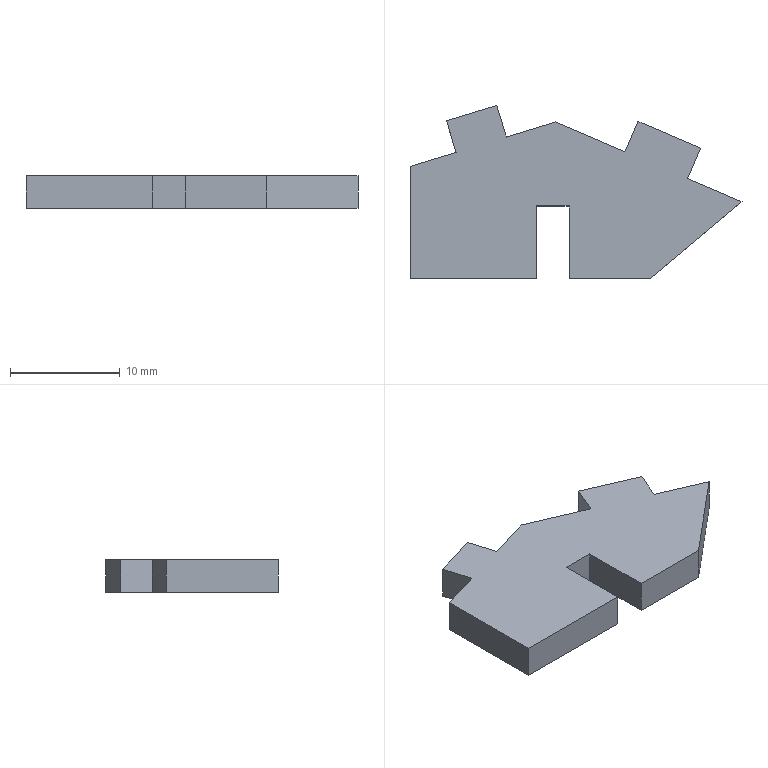Part | SolidWorks | features BaseBody 1 | 1 solid | 19 faces | box 30.19 x 15.728 x 3 mm | volume 976.477 mm3 | plane 19
STEP:
#1=CARTESIAN_POINT('',(14.396,15.946,-1.5));
#2=VERTEX_POINT('',#1);
#3=CARTESIAN_POINT('',(14.396,5.749,-1.5));
#4=VERTEX_POINT('',#3);
#5=CARTESIAN_POINT('',(14.396,15.946,-1.5));
#6=DIRECTION('',(0.,-1.,0.));
#7=VECTOR('',#6,1000.);
#8=LINE('',#5,#7);
#9=EDGE_CURVE('',#2,#4,#8,.T.);
#10=ORIENTED_EDGE('',*,*,#9,.F.);
#11=CARTESIAN_POINT('',(18.585,17.221,-1.5));
#12=VERTEX_POINT('',#11);
#13=CARTESIAN_POINT('',(18.585,17.221,-1.5));
#14=DIRECTION('',(-0.9567,-0.2912,0.));
#15=VECTOR('',#14,1000.);
#16=LINE('',#13,#15);
#17=EDGE_CURVE('',#12,#2,#16,.T.);
#18=ORIENTED_EDGE('',*,*,#17,.F.);
#19=CARTESIAN_POINT('',(17.713,20.086,-1.5));
#20=VERTEX_POINT('',#19);
#21=CARTESIAN_POINT('',(17.713,20.086,-1.5));
#22=DIRECTION('',(0.2911,-0.9567,0.));
#23=VECTOR('',#22,1000.);
#24=LINE('',#21,#23);
#25=EDGE_CURVE('',#20,#12,#24,.T.);
#26=ORIENTED_EDGE('',*,*,#25,.F.);
#27=CARTESIAN_POINT('',(22.284,21.477,-1.5));
#28=VERTEX_POINT('',#27);
#29=CARTESIAN_POINT('',(22.284,21.477,-1.5));
#30=DIRECTION('',(-0.9567,-0.2911,0.));
#31=VECTOR('',#30,1000.);
#32=LINE('',#29,#31);
#33=EDGE_CURVE('',#28,#20,#32,.T.);
#34=ORIENTED_EDGE('',*,*,#33,.F.);
#35=CARTESIAN_POINT('',(23.157,18.609,-1.5));
#36=VERTEX_POINT('',#35);
#37=CARTESIAN_POINT('',(23.157,18.609,-1.5));
#38=DIRECTION('',(-0.2911,0.9567,0.));
#39=VECTOR('',#38,1000.);
#40=LINE('',#37,#39);
#41=EDGE_CURVE('',#36,#28,#40,.T.);
#42=ORIENTED_EDGE('',*,*,#41,.F.);
#43=CARTESIAN_POINT('',(27.665,19.98,-1.5));
#44=VERTEX_POINT('',#43);
#45=CARTESIAN_POINT('',(27.665,19.98,-1.5));
#46=DIRECTION('',(-0.9567,-0.2909,0.));
#47=VECTOR('',#46,1000.);
#48=LINE('',#45,#47);
#49=EDGE_CURVE('',#44,#36,#48,.T.);
#50=ORIENTED_EDGE('',*,*,#49,.F.);
#51=CARTESIAN_POINT('',(33.945,17.285,-1.5));
#52=VERTEX_POINT('',#51);
#53=CARTESIAN_POINT('',(33.945,17.285,-1.5));
#54=DIRECTION('',(-0.9189,0.3944,0.));
#55=VECTOR('',#54,1000.);
#56=LINE('',#53,#55);
#57=EDGE_CURVE('',#52,#44,#56,.T.);
#58=ORIENTED_EDGE('',*,*,#57,.F.);
#59=CARTESIAN_POINT('',(35.126,20.04,-1.5));
#60=VERTEX_POINT('',#59);
#61=CARTESIAN_POINT('',(35.126,20.04,-1.5));
#62=DIRECTION('',(-0.3942,-0.919,0.));
#63=VECTOR('',#62,1000.);
#64=LINE('',#61,#63);
#65=EDGE_CURVE('',#60,#52,#64,.T.);
#66=ORIENTED_EDGE('',*,*,#65,.F.);
#67=CARTESIAN_POINT('',(40.814,17.6,-1.5));
#68=VERTEX_POINT('',#67);
#69=CARTESIAN_POINT('',(40.814,17.6,-1.5));
#70=DIRECTION('',(-0.919,0.3942,0.));
#71=VECTOR('',#70,1000.);
#72=LINE('',#69,#71);
#73=EDGE_CURVE('',#68,#60,#72,.T.);
#74=ORIENTED_EDGE('',*,*,#73,.F.);
#75=CARTESIAN_POINT('',(39.633,14.845,-1.5));
#76=VERTEX_POINT('',#75);
#77=CARTESIAN_POINT('',(39.633,14.845,-1.5));
#78=DIRECTION('',(0.3942,0.919,0.));
#79=VECTOR('',#78,1000.);
#80=LINE('',#77,#79);
#81=EDGE_CURVE('',#76,#68,#80,.T.);
#82=ORIENTED_EDGE('',*,*,#81,.F.);
#83=CARTESIAN_POINT('',(44.585,12.721,-1.5));
#84=VERTEX_POINT('',#83);
#85=CARTESIAN_POINT('',(44.585,12.721,-1.5));
#86=DIRECTION('',(-0.919,0.3942,0.));
#87=VECTOR('',#86,1000.);
#88=LINE('',#85,#87);
#89=EDGE_CURVE('',#84,#76,#88,.T.);
#90=ORIENTED_EDGE('',*,*,#89,.F.);
#91=CARTESIAN_POINT('',(36.243,5.749,-1.5));
#92=VERTEX_POINT('',#91);
#93=CARTESIAN_POINT('',(36.243,5.749,-1.5));
#94=DIRECTION('',(0.7673,0.6413,0.));
#95=VECTOR('',#94,1000.);
#96=LINE('',#93,#95);
#97=EDGE_CURVE('',#92,#84,#96,.T.);
#98=ORIENTED_EDGE('',*,*,#97,.F.);
#99=CARTESIAN_POINT('',(28.864,5.749,-1.5));
#100=VERTEX_POINT('',#99);
#101=CARTESIAN_POINT('',(28.864,5.749,-1.5));
#102=DIRECTION('',(1.,0.,0.));
#103=VECTOR('',#102,1000.);
#104=LINE('',#101,#103);
#105=EDGE_CURVE('',#100,#92,#104,.T.);
#106=ORIENTED_EDGE('',*,*,#105,.F.);
#107=CARTESIAN_POINT('',(28.864,12.338,-1.5));
#108=VERTEX_POINT('',#107);
#109=CARTESIAN_POINT('',(28.864,12.338,-1.5));
#110=DIRECTION('',(0.,-1.,0.));
#111=VECTOR('',#110,1000.);
#112=LINE('',#109,#111);
#113=EDGE_CURVE('',#108,#100,#112,.T.);
#114=ORIENTED_EDGE('',*,*,#113,.F.);
#115=CARTESIAN_POINT('',(25.869,12.338,-1.5));
#116=VERTEX_POINT('',#115);
#117=CARTESIAN_POINT('',(25.869,12.338,-1.5));
#118=DIRECTION('',(1.,0.,0.));
#119=VECTOR('',#118,1000.);
#120=LINE('',#117,#119);
#121=EDGE_CURVE('',#116,#108,#120,.T.);
#122=ORIENTED_EDGE('',*,*,#121,.F.);
#123=CARTESIAN_POINT('',(25.869,5.749,-1.5));
#124=VERTEX_POINT('',#123);
#125=CARTESIAN_POINT('',(25.869,5.749,-1.5));
#126=DIRECTION('',(0.,1.,0.));
#127=VECTOR('',#126,1000.);
#128=LINE('',#125,#127);
#129=EDGE_CURVE('',#124,#116,#128,.T.);
#130=ORIENTED_EDGE('',*,*,#129,.F.);
#131=CARTESIAN_POINT('',(14.396,5.749,-1.5));
#132=DIRECTION('',(1.,0.,0.));
#133=VECTOR('',#132,1000.);
#134=LINE('',#131,#133);
#135=EDGE_CURVE('',#4,#124,#134,.T.);
#136=ORIENTED_EDGE('',*,*,#135,.F.);
#137=EDGE_LOOP('',(#10,#18,#26,#34,#42,#50,#58,#66,#74,#82,#90,#98,#106,#114,#122,#130,#136));
#138=FACE_OUTER_BOUND('',#137,.T.);
#139=CARTESIAN_POINT('',(0.,0.,-1.5));
#140=DIRECTION('',(0.,0.,1.));
#141=DIRECTION('',(1.,0.,0.));
#142=AXIS2_PLACEMENT_3D('',#139,#140,#141);
#143=PLANE('',#142);
#144=ADVANCED_FACE('',(#138),#143,.F.);
#145=CARTESIAN_POINT('',(14.396,15.946,1.5));
#146=VERTEX_POINT('',#145);
#147=CARTESIAN_POINT('',(14.396,5.749,1.5));
#148=VERTEX_POINT('',#147);
#149=CARTESIAN_POINT('',(14.396,15.946,1.5));
#150=DIRECTION('',(0.,-1.,0.));
#151=VECTOR('',#150,1000.);
#152=LINE('',#149,#151);
#153=EDGE_CURVE('',#146,#148,#152,.T.);
#154=ORIENTED_EDGE('',*,*,#153,.T.);
#155=CARTESIAN_POINT('',(25.869,5.749,1.5));
#156=VERTEX_POINT('',#155);
#157=CARTESIAN_POINT('',(14.396,5.749,1.5));
#158=DIRECTION('',(1.,0.,0.));
#159=VECTOR('',#158,1000.);
#160=LINE('',#157,#159);
#161=EDGE_CURVE('',#148,#156,#160,.T.);
#162=ORIENTED_EDGE('',*,*,#161,.T.);
#163=CARTESIAN_POINT('',(25.869,12.338,1.5));
#164=VERTEX_POINT('',#163);
#165=CARTESIAN_POINT('',(25.869,5.749,1.5));
#166=DIRECTION('',(0.,1.,0.));
#167=VECTOR('',#166,1000.);
#168=LINE('',#165,#167);
#169=EDGE_CURVE('',#156,#164,#168,.T.);
#170=ORIENTED_EDGE('',*,*,#169,.T.);
#171=CARTESIAN_POINT('',(28.864,12.338,1.5));
#172=VERTEX_POINT('',#171);
#173=CARTESIAN_POINT('',(25.869,12.338,1.5));
#174=DIRECTION('',(1.,0.,0.));
#175=VECTOR('',#174,1000.);
#176=LINE('',#173,#175);
#177=EDGE_CURVE('',#164,#172,#176,.T.);
#178=ORIENTED_EDGE('',*,*,#177,.T.);
#179=CARTESIAN_POINT('',(28.864,5.749,1.5));
#180=VERTEX_POINT('',#179);
#181=CARTESIAN_POINT('',(28.864,12.338,1.5));
#182=DIRECTION('',(0.,-1.,0.));
#183=VECTOR('',#182,1000.);
#184=LINE('',#181,#183);
#185=EDGE_CURVE('',#172,#180,#184,.T.);
#186=ORIENTED_EDGE('',*,*,#185,.T.);
#187=CARTESIAN_POINT('',(36.243,5.749,1.5));
#188=VERTEX_POINT('',#187);
#189=CARTESIAN_POINT('',(28.864,5.749,1.5));
#190=DIRECTION('',(1.,0.,0.));
#191=VECTOR('',#190,1000.);
#192=LINE('',#189,#191);
#193=EDGE_CURVE('',#180,#188,#192,.T.);
#194=ORIENTED_EDGE('',*,*,#193,.T.);
#195=CARTESIAN_POINT('',(44.585,12.721,1.5));
#196=VERTEX_POINT('',#195);
#197=CARTESIAN_POINT('',(36.243,5.749,1.5));
#198=DIRECTION('',(0.7673,0.6413,0.));
#199=VECTOR('',#198,1000.);
#200=LINE('',#197,#199);
#201=EDGE_CURVE('',#188,#196,#200,.T.);
#202=ORIENTED_EDGE('',*,*,#201,.T.);
#203=CARTESIAN_POINT('',(39.633,14.845,1.5));
#204=VERTEX_POINT('',#203);
#205=CARTESIAN_POINT('',(44.585,12.721,1.5));
#206=DIRECTION('',(-0.919,0.3942,0.));
#207=VECTOR('',#206,1000.);
#208=LINE('',#205,#207);
#209=EDGE_CURVE('',#196,#204,#208,.T.);
#210=ORIENTED_EDGE('',*,*,#209,.T.);
#211=CARTESIAN_POINT('',(40.814,17.6,1.5));
#212=VERTEX_POINT('',#211);
#213=CARTESIAN_POINT('',(39.633,14.845,1.5));
#214=DIRECTION('',(0.3942,0.919,0.));
#215=VECTOR('',#214,1000.);
#216=LINE('',#213,#215);
#217=EDGE_CURVE('',#204,#212,#216,.T.);
#218=ORIENTED_EDGE('',*,*,#217,.T.);
#219=CARTESIAN_POINT('',(35.126,20.04,1.5));
#220=VERTEX_POINT('',#219);
#221=CARTESIAN_POINT('',(40.814,17.6,1.5));
#222=DIRECTION('',(-0.919,0.3942,0.));
#223=VECTOR('',#222,1000.);
#224=LINE('',#221,#223);
#225=EDGE_CURVE('',#212,#220,#224,.T.);
#226=ORIENTED_EDGE('',*,*,#225,.T.);
#227=CARTESIAN_POINT('',(33.945,17.285,1.5));
#228=VERTEX_POINT('',#227);
#229=CARTESIAN_POINT('',(35.126,20.04,1.5));
#230=DIRECTION('',(-0.3942,-0.919,0.));
#231=VECTOR('',#230,1000.);
#232=LINE('',#229,#231);
#233=EDGE_CURVE('',#220,#228,#232,.T.);
#234=ORIENTED_EDGE('',*,*,#233,.T.);
#235=CARTESIAN_POINT('',(27.665,19.98,1.5));
#236=VERTEX_POINT('',#235);
#237=CARTESIAN_POINT('',(33.945,17.285,1.5));
#238=DIRECTION('',(-0.9189,0.3944,0.));
#239=VECTOR('',#238,1000.);
#240=LINE('',#237,#239);
#241=EDGE_CURVE('',#228,#236,#240,.T.);
#242=ORIENTED_EDGE('',*,*,#241,.T.);
#243=CARTESIAN_POINT('',(23.157,18.609,1.5));
#244=VERTEX_POINT('',#243);
#245=CARTESIAN_POINT('',(27.665,19.98,1.5));
#246=DIRECTION('',(-0.9567,-0.2909,0.));
#247=VECTOR('',#246,1000.);
#248=LINE('',#245,#247);
#249=EDGE_CURVE('',#236,#244,#248,.T.);
#250=ORIENTED_EDGE('',*,*,#249,.T.);
#251=CARTESIAN_POINT('',(22.284,21.477,1.5));
#252=VERTEX_POINT('',#251);
#253=CARTESIAN_POINT('',(23.157,18.609,1.5));
#254=DIRECTION('',(-0.2911,0.9567,0.));
#255=VECTOR('',#254,1000.);
#256=LINE('',#253,#255);
#257=EDGE_CURVE('',#244,#252,#256,.T.);
#258=ORIENTED_EDGE('',*,*,#257,.T.);
#259=CARTESIAN_POINT('',(17.713,20.086,1.5));
#260=VERTEX_POINT('',#259);
#261=CARTESIAN_POINT('',(22.284,21.477,1.5));
#262=DIRECTION('',(-0.9567,-0.2911,0.));
#263=VECTOR('',#262,1000.);
#264=LINE('',#261,#263);
#265=EDGE_CURVE('',#252,#260,#264,.T.);
#266=ORIENTED_EDGE('',*,*,#265,.T.);
#267=CARTESIAN_POINT('',(18.585,17.221,1.5));
#268=VERTEX_POINT('',#267);
#269=CARTESIAN_POINT('',(17.713,20.086,1.5));
#270=DIRECTION('',(0.2911,-0.9567,0.));
#271=VECTOR('',#270,1000.);
#272=LINE('',#269,#271);
#273=EDGE_CURVE('',#260,#268,#272,.T.);
#274=ORIENTED_EDGE('',*,*,#273,.T.);
#275=CARTESIAN_POINT('',(18.585,17.221,1.5));
#276=DIRECTION('',(-0.9567,-0.2912,0.));
#277=VECTOR('',#276,1000.);
#278=LINE('',#275,#277);
#279=EDGE_CURVE('',#268,#146,#278,.T.);
#280=ORIENTED_EDGE('',*,*,#279,.T.);
#281=EDGE_LOOP('',(#154,#162,#170,#178,#186,#194,#202,#210,#218,#226,#234,#242,#250,#258,#266,#274,#280));
#282=FACE_OUTER_BOUND('',#281,.T.);
#283=CARTESIAN_POINT('',(0.,0.,1.5));
#284=DIRECTION('',(0.,0.,1.));
#285=DIRECTION('',(1.,0.,0.));
#286=AXIS2_PLACEMENT_3D('',#283,#284,#285);
#287=PLANE('',#286);
#288=ADVANCED_FACE('',(#282),#287,.T.);
#289=ORIENTED_EDGE('',*,*,#17,.T.);
#290=CARTESIAN_POINT('',(14.396,15.946,1.5));
#291=DIRECTION('',(0.,0.,-1.));
#292=VECTOR('',#291,1000.);
#293=LINE('',#290,#292);
#294=EDGE_CURVE('',#146,#2,#293,.T.);
#295=ORIENTED_EDGE('',*,*,#294,.F.);
#296=ORIENTED_EDGE('',*,*,#279,.F.);
#297=CARTESIAN_POINT('',(18.585,17.221,1.5));
#298=DIRECTION('',(0.,0.,-1.));
#299=VECTOR('',#298,1000.);
#300=LINE('',#297,#299);
#301=EDGE_CURVE('',#268,#12,#300,.T.);
#302=ORIENTED_EDGE('',*,*,#301,.T.);
#303=EDGE_LOOP('',(#289,#295,#296,#302));
#304=FACE_OUTER_BOUND('',#303,.T.);
#305=CARTESIAN_POINT('',(18.585,17.221,1.5));
#306=DIRECTION('',(0.2912,-0.9567,0.));
#307=DIRECTION('',(0.,0.,-1.));
#308=AXIS2_PLACEMENT_3D('',#305,#306,#307);
#309=PLANE('',#308);
#310=ADVANCED_FACE('',(#304),#309,.F.);
#311=ORIENTED_EDGE('',*,*,#25,.T.);
#312=ORIENTED_EDGE('',*,*,#301,.F.);
#313=ORIENTED_EDGE('',*,*,#273,.F.);
#314=CARTESIAN_POINT('',(17.713,20.086,1.5));
#315=DIRECTION('',(0.,0.,-1.));
#316=VECTOR('',#315,1000.);
#317=LINE('',#314,#316);
#318=EDGE_CURVE('',#260,#20,#317,.T.);
#319=ORIENTED_EDGE('',*,*,#318,.T.);
#320=EDGE_LOOP('',(#311,#312,#313,#319));
#321=FACE_OUTER_BOUND('',#320,.T.);
#322=CARTESIAN_POINT('',(17.713,20.086,1.5));
#323=DIRECTION('',(0.9567,0.2911,0.));
#324=DIRECTION('',(0.,0.,-1.));
#325=AXIS2_PLACEMENT_3D('',#322,#323,#324);
#326=PLANE('',#325);
#327=ADVANCED_FACE('',(#321),#326,.F.);
#328=ORIENTED_EDGE('',*,*,#33,.T.);
#329=ORIENTED_EDGE('',*,*,#318,.F.);
#330=ORIENTED_EDGE('',*,*,#265,.F.);
#331=CARTESIAN_POINT('',(22.284,21.477,1.5));
#332=DIRECTION('',(0.,0.,-1.));
#333=VECTOR('',#332,1000.);
#334=LINE('',#331,#333);
#335=EDGE_CURVE('',#252,#28,#334,.T.);
#336=ORIENTED_EDGE('',*,*,#335,.T.);
#337=EDGE_LOOP('',(#328,#329,#330,#336));
#338=FACE_OUTER_BOUND('',#337,.T.);
#339=CARTESIAN_POINT('',(22.284,21.477,1.5));
#340=DIRECTION('',(0.2911,-0.9567,0.));
#341=DIRECTION('',(0.,0.,-1.));
#342=AXIS2_PLACEMENT_3D('',#339,#340,#341);
#343=PLANE('',#342);
#344=ADVANCED_FACE('',(#338),#343,.F.);
#345=ORIENTED_EDGE('',*,*,#41,.T.);
#346=ORIENTED_EDGE('',*,*,#335,.F.);
#347=ORIENTED_EDGE('',*,*,#257,.F.);
#348=CARTESIAN_POINT('',(23.157,18.609,1.5));
#349=DIRECTION('',(0.,0.,-1.));
#350=VECTOR('',#349,1000.);
#351=LINE('',#348,#350);
#352=EDGE_CURVE('',#244,#36,#351,.T.);
#353=ORIENTED_EDGE('',*,*,#352,.T.);
#354=EDGE_LOOP('',(#345,#346,#347,#353));
#355=FACE_OUTER_BOUND('',#354,.T.);
#356=CARTESIAN_POINT('',(23.157,18.609,1.5));
#357=DIRECTION('',(-0.9567,-0.2911,0.));
#358=DIRECTION('',(-0.2911,0.9567,0.));
#359=AXIS2_PLACEMENT_3D('',#356,#357,#358);
#360=PLANE('',#359);
#361=ADVANCED_FACE('',(#355),#360,.F.);
#362=ORIENTED_EDGE('',*,*,#49,.T.);
#363=ORIENTED_EDGE('',*,*,#352,.F.);
#364=ORIENTED_EDGE('',*,*,#249,.F.);
#365=CARTESIAN_POINT('',(27.665,19.98,1.5));
#366=DIRECTION('',(0.,0.,-1.));
#367=VECTOR('',#366,1000.);
#368=LINE('',#365,#367);
#369=EDGE_CURVE('',#236,#44,#368,.T.);
#370=ORIENTED_EDGE('',*,*,#369,.T.);
#371=EDGE_LOOP('',(#362,#363,#364,#370));
#372=FACE_OUTER_BOUND('',#371,.T.);
#373=CARTESIAN_POINT('',(27.665,19.98,1.5));
#374=DIRECTION('',(0.2909,-0.9567,0.));
#375=DIRECTION('',(0.,0.,-1.));
#376=AXIS2_PLACEMENT_3D('',#373,#374,#375);
#377=PLANE('',#376);
#378=ADVANCED_FACE('',(#372),#377,.F.);
#379=ORIENTED_EDGE('',*,*,#57,.T.);
#380=ORIENTED_EDGE('',*,*,#369,.F.);
#381=ORIENTED_EDGE('',*,*,#241,.F.);
#382=CARTESIAN_POINT('',(33.945,17.285,1.5));
#383=DIRECTION('',(0.,0.,-1.));
#384=VECTOR('',#383,1000.);
#385=LINE('',#382,#384);
#386=EDGE_CURVE('',#228,#52,#385,.T.);
#387=ORIENTED_EDGE('',*,*,#386,.T.);
#388=EDGE_LOOP('',(#379,#380,#381,#387));
#389=FACE_OUTER_BOUND('',#388,.T.);
#390=CARTESIAN_POINT('',(33.945,17.285,1.5));
#391=DIRECTION('',(-0.3944,-0.9189,0.));
#392=DIRECTION('',(-0.9189,0.3944,0.));
#393=AXIS2_PLACEMENT_3D('',#390,#391,#392);
#394=PLANE('',#393);
#395=ADVANCED_FACE('',(#389),#394,.F.);
#396=ORIENTED_EDGE('',*,*,#65,.T.);
#397=ORIENTED_EDGE('',*,*,#386,.F.);
#398=ORIENTED_EDGE('',*,*,#233,.F.);
#399=CARTESIAN_POINT('',(35.126,20.04,1.5));
#400=DIRECTION('',(0.,0.,-1.));
#401=VECTOR('',#400,1000.);
#402=LINE('',#399,#401);
#403=EDGE_CURVE('',#220,#60,#402,.T.);
#404=ORIENTED_EDGE('',*,*,#403,.T.);
#405=EDGE_LOOP('',(#396,#397,#398,#404));
#406=FACE_OUTER_BOUND('',#405,.T.);
#407=CARTESIAN_POINT('',(35.126,20.04,1.5));
#408=DIRECTION('',(0.919,-0.3942,0.));
#409=DIRECTION('',(0.,0.,-1.));
#410=AXIS2_PLACEMENT_3D('',#407,#408,#409);
#411=PLANE('',#410);
#412=ADVANCED_FACE('',(#406),#411,.F.);
#413=ORIENTED_EDGE('',*,*,#73,.T.);
#414=ORIENTED_EDGE('',*,*,#403,.F.);
#415=ORIENTED_EDGE('',*,*,#225,.F.);
#416=CARTESIAN_POINT('',(40.814,17.6,1.5));
#417=DIRECTION('',(0.,0.,-1.));
#418=VECTOR('',#417,1000.);
#419=LINE('',#416,#418);
#420=EDGE_CURVE('',#212,#68,#419,.T.);
#421=ORIENTED_EDGE('',*,*,#420,.T.);
#422=EDGE_LOOP('',(#413,#414,#415,#421));
#423=FACE_OUTER_BOUND('',#422,.T.);
#424=CARTESIAN_POINT('',(40.814,17.6,1.5));
#425=DIRECTION('',(-0.3942,-0.919,0.));
#426=DIRECTION('',(-0.919,0.3942,0.));
#427=AXIS2_PLACEMENT_3D('',#424,#425,#426);
#428=PLANE('',#427);
#429=ADVANCED_FACE('',(#423),#428,.F.);
#430=ORIENTED_EDGE('',*,*,#81,.T.);
#431=ORIENTED_EDGE('',*,*,#420,.F.);
#432=ORIENTED_EDGE('',*,*,#217,.F.);
#433=CARTESIAN_POINT('',(39.633,14.845,1.5));
#434=DIRECTION('',(0.,0.,-1.));
#435=VECTOR('',#434,1000.);
#436=LINE('',#433,#435);
#437=EDGE_CURVE('',#204,#76,#436,.T.);
#438=ORIENTED_EDGE('',*,*,#437,.T.);
#439=EDGE_LOOP('',(#430,#431,#432,#438));
#440=FACE_OUTER_BOUND('',#439,.T.);
#441=CARTESIAN_POINT('',(39.633,14.845,1.5));
#442=DIRECTION('',(-0.919,0.3942,0.));
#443=DIRECTION('',(0.,0.,1.));
#444=AXIS2_PLACEMENT_3D('',#441,#442,#443);
#445=PLANE('',#444);
#446=ADVANCED_FACE('',(#440),#445,.F.);
#447=ORIENTED_EDGE('',*,*,#89,.T.);
#448=ORIENTED_EDGE('',*,*,#437,.F.);
#449=ORIENTED_EDGE('',*,*,#209,.F.);
#450=CARTESIAN_POINT('',(44.585,12.721,1.5));
#451=DIRECTION('',(0.,0.,-1.));
#452=VECTOR('',#451,1000.);
#453=LINE('',#450,#452);
#454=EDGE_CURVE('',#196,#84,#453,.T.);
#455=ORIENTED_EDGE('',*,*,#454,.T.);
#456=EDGE_LOOP('',(#447,#448,#449,#455));
#457=FACE_OUTER_BOUND('',#456,.T.);
#458=CARTESIAN_POINT('',(44.585,12.721,1.5));
#459=DIRECTION('',(-0.3942,-0.919,0.));
#460=DIRECTION('',(-0.919,0.3942,0.));
#461=AXIS2_PLACEMENT_3D('',#458,#459,#460);
#462=PLANE('',#461);
#463=ADVANCED_FACE('',(#457),#462,.F.);
#464=ORIENTED_EDGE('',*,*,#97,.T.);
#465=ORIENTED_EDGE('',*,*,#454,.F.);
#466=ORIENTED_EDGE('',*,*,#201,.F.);
#467=CARTESIAN_POINT('',(36.243,5.749,1.5));
#468=DIRECTION('',(0.,0.,-1.));
#469=VECTOR('',#468,1000.);
#470=LINE('',#467,#469);
#471=EDGE_CURVE('',#188,#92,#470,.T.);
#472=ORIENTED_EDGE('',*,*,#471,.T.);
#473=EDGE_LOOP('',(#464,#465,#466,#472));
#474=FACE_OUTER_BOUND('',#473,.T.);
#475=CARTESIAN_POINT('',(36.243,5.749,1.5));
#476=DIRECTION('',(-0.6413,0.7673,0.));
#477=DIRECTION('',(0.,0.,1.));
#478=AXIS2_PLACEMENT_3D('',#475,#476,#477);
#479=PLANE('',#478);
#480=ADVANCED_FACE('',(#474),#479,.F.);
#481=ORIENTED_EDGE('',*,*,#105,.T.);
#482=ORIENTED_EDGE('',*,*,#471,.F.);
#483=ORIENTED_EDGE('',*,*,#193,.F.);
#484=CARTESIAN_POINT('',(28.864,5.749,1.5));
#485=DIRECTION('',(0.,0.,-1.));
#486=VECTOR('',#485,1000.);
#487=LINE('',#484,#486);
#488=EDGE_CURVE('',#180,#100,#487,.T.);
#489=ORIENTED_EDGE('',*,*,#488,.T.);
#490=EDGE_LOOP('',(#481,#482,#483,#489));
#491=FACE_OUTER_BOUND('',#490,.T.);
#492=CARTESIAN_POINT('',(28.864,5.749,1.5));
#493=DIRECTION('',(0.,1.,0.));
#494=DIRECTION('',(1.,0.,0.));
#495=AXIS2_PLACEMENT_3D('',#492,#493,#494);
#496=PLANE('',#495);
#497=ADVANCED_FACE('',(#491),#496,.F.);
#498=ORIENTED_EDGE('',*,*,#113,.T.);
#499=ORIENTED_EDGE('',*,*,#488,.F.);
#500=ORIENTED_EDGE('',*,*,#185,.F.);
#501=CARTESIAN_POINT('',(28.864,12.338,1.5));
#502=DIRECTION('',(0.,0.,-1.));
#503=VECTOR('',#502,1000.);
#504=LINE('',#501,#503);
#505=EDGE_CURVE('',#172,#108,#504,.T.);
#506=ORIENTED_EDGE('',*,*,#505,.T.);
#507=EDGE_LOOP('',(#498,#499,#500,#506));
#508=FACE_OUTER_BOUND('',#507,.T.);
#509=CARTESIAN_POINT('',(28.864,12.338,1.5));
#510=DIRECTION('',(1.,0.,0.));
#511=DIRECTION('',(0.,1.,0.));
#512=AXIS2_PLACEMENT_3D('',#509,#510,#511);
#513=PLANE('',#512);
#514=ADVANCED_FACE('',(#508),#513,.F.);
#515=ORIENTED_EDGE('',*,*,#121,.T.);
#516=ORIENTED_EDGE('',*,*,#505,.F.);
#517=ORIENTED_EDGE('',*,*,#177,.F.);
#518=CARTESIAN_POINT('',(25.869,12.338,1.5));
#519=DIRECTION('',(0.,0.,-1.));
#520=VECTOR('',#519,1000.);
#521=LINE('',#518,#520);
#522=EDGE_CURVE('',#164,#116,#521,.T.);
#523=ORIENTED_EDGE('',*,*,#522,.T.);
#524=EDGE_LOOP('',(#515,#516,#517,#523));
#525=FACE_OUTER_BOUND('',#524,.T.);
#526=CARTESIAN_POINT('',(25.869,12.338,1.5));
#527=DIRECTION('',(0.,1.,0.));
#528=DIRECTION('',(1.,0.,0.));
#529=AXIS2_PLACEMENT_3D('',#526,#527,#528);
#530=PLANE('',#529);
#531=ADVANCED_FACE('',(#525),#530,.F.);
#532=ORIENTED_EDGE('',*,*,#129,.T.);
#533=ORIENTED_EDGE('',*,*,#522,.F.);
#534=ORIENTED_EDGE('',*,*,#169,.F.);
#535=CARTESIAN_POINT('',(25.869,5.749,1.5));
#536=DIRECTION('',(0.,0.,-1.));
#537=VECTOR('',#536,1000.);
#538=LINE('',#535,#537);
#539=EDGE_CURVE('',#156,#124,#538,.T.);
#540=ORIENTED_EDGE('',*,*,#539,.T.);
#541=EDGE_LOOP('',(#532,#533,#534,#540));
#542=FACE_OUTER_BOUND('',#541,.T.);
#543=CARTESIAN_POINT('',(25.869,5.749,1.5));
#544=DIRECTION('',(-1.,0.,0.));
#545=DIRECTION('',(0.,0.,1.));
#546=AXIS2_PLACEMENT_3D('',#543,#544,#545);
#547=PLANE('',#546);
#548=ADVANCED_FACE('',(#542),#547,.F.);
#549=ORIENTED_EDGE('',*,*,#135,.T.);
#550=ORIENTED_EDGE('',*,*,#539,.F.);
#551=ORIENTED_EDGE('',*,*,#161,.F.);
#552=CARTESIAN_POINT('',(14.396,5.749,1.5));
#553=DIRECTION('',(0.,0.,-1.));
#554=VECTOR('',#553,1000.);
#555=LINE('',#552,#554);
#556=EDGE_CURVE('',#148,#4,#555,.T.);
#557=ORIENTED_EDGE('',*,*,#556,.T.);
#558=EDGE_LOOP('',(#549,#550,#551,#557));
#559=FACE_OUTER_BOUND('',#558,.T.);
#560=CARTESIAN_POINT('',(14.396,5.749,1.5));
#561=DIRECTION('',(0.,1.,0.));
#562=DIRECTION('',(1.,0.,0.));
#563=AXIS2_PLACEMENT_3D('',#560,#561,#562);
#564=PLANE('',#563);
#565=ADVANCED_FACE('',(#559),#564,.F.);
#566=ORIENTED_EDGE('',*,*,#9,.T.);
#567=ORIENTED_EDGE('',*,*,#556,.F.);
#568=ORIENTED_EDGE('',*,*,#153,.F.);
#569=ORIENTED_EDGE('',*,*,#294,.T.);
#570=EDGE_LOOP('',(#566,#567,#568,#569));
#571=FACE_OUTER_BOUND('',#570,.T.);
#572=CARTESIAN_POINT('',(14.396,15.946,1.5));
#573=DIRECTION('',(1.,0.,0.));
#574=DIRECTION('',(0.,1.,0.));
#575=AXIS2_PLACEMENT_3D('',#572,#573,#574);
#576=PLANE('',#575);
#577=ADVANCED_FACE('',(#571),#576,.F.);
#578=CLOSED_SHELL('',(#144,#288,#310,#327,#344,#361,#378,#395,#412,#429,#446,#463,#480,#497,#514,#531,#548,#565,#577));
#579=MANIFOLD_SOLID_BREP('',#578);
#580=CARTESIAN_POINT('',(0.,0.,0.));
#581=DIRECTION('',(0.,0.,1.));
#582=DIRECTION('',(1.,0.,0.));
#583=AXIS2_PLACEMENT_3D('',#580,#581,#582);
#584=(LENGTH_UNIT()NAMED_UNIT(*)SI_UNIT(.MILLI.,.METRE.));
#585=UNCERTAINTY_MEASURE_WITH_UNIT(LENGTH_MEASURE(0.00001),#584,'','');
#586=(NAMED_UNIT(*)PLANE_ANGLE_UNIT()SI_UNIT($,.RADIAN.));
#587=(NAMED_UNIT(*)SI_UNIT($,.STERADIAN.)SOLID_ANGLE_UNIT());
#588=(GEOMETRIC_REPRESENTATION_CONTEXT(3)GLOBAL_UNCERTAINTY_ASSIGNED_CONTEXT((#585))GLOBAL_UNIT_ASSIGNED_CONTEXT((#584,#586,#587))REPRESENTATION_CONTEXT('',''));
#589=ADVANCED_BREP_SHAPE_REPRESENTATION('',(#579,#583),#588);